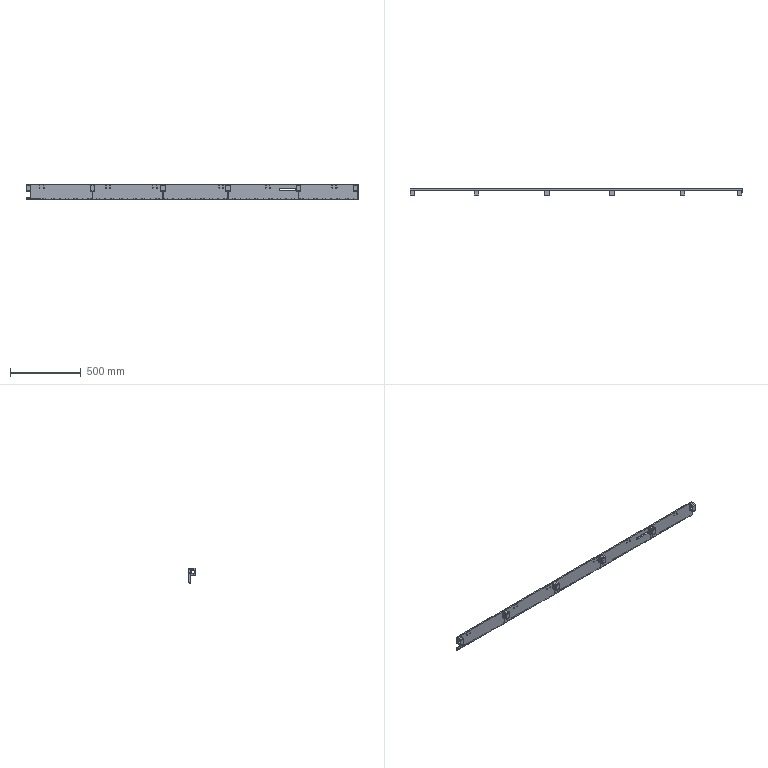Part | NX | 11 solids | 1206 faces | box 2350 x 45.7 x 110 mm | volume 2646245 mm3 | cylinder 496 | cone 475 | plane 235 | commonest cylinder face diameters 4.2 x216 3.3 x88 4 x70 2.5 x48 5.5 x48 25 x12